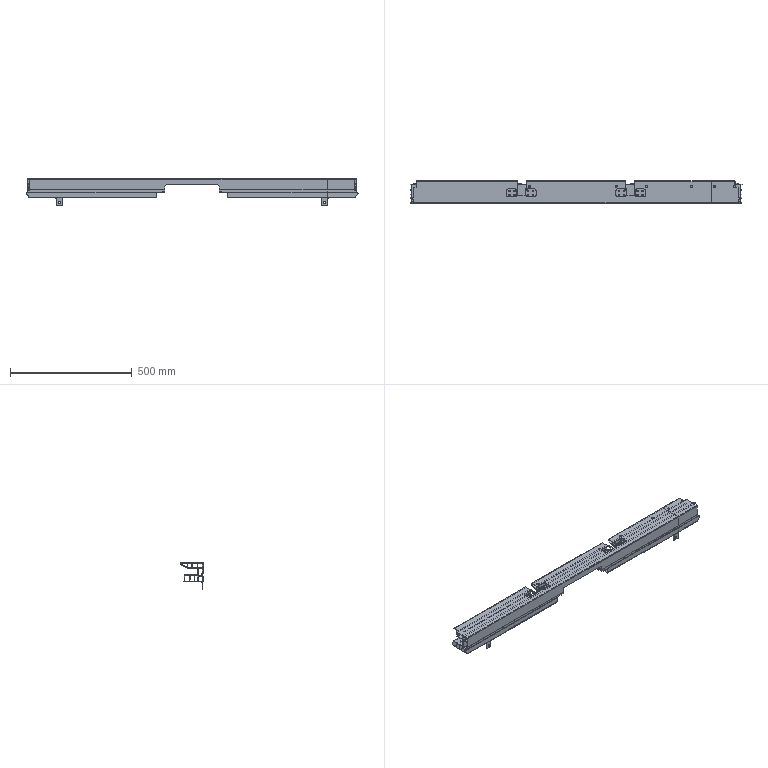NC program | NX | posted with a generic post | part box 1365 x 90.95 x 108.501 mm
Lines 1 to 35 of 25066:
N10 G17 G21 G94 G90
(DRILLING_1 , TOOL : D6A45)
N12 T07 M6
N14 G54
N16 G17 G0 G90 X191.807 Y-23.125 B0. C0. S3500 M3
N18 G43 Z30. H7
N20 G94 G81 G98 Z-1.001 F250. R2.999
N22 X-165.096
N24 X-290.143
N26 X-475.
N28 X-570.
N30 X-652.
N32 G80
N34 G0 X-652. Y-23.125 Z30.
N36 M5
(DRILLING_COPY_3 , TOOL : 8.1ZT)
N38 T18 M6
N40 G54
N42 G17 G0 G90 X191.807 Y-23.125 B0. C0. S1500 M3
N44 G43 Z30. H18
N46 G94 G83 G98 Z-54.405 F150. Q4. R2.999
N48 X-165.096
N50 X-290.143
N52 X-475.
N54 X-570.
N56 X-652.
N58 G80
N60 G0 X-652. Y-23.125 Z30.
N62 M5